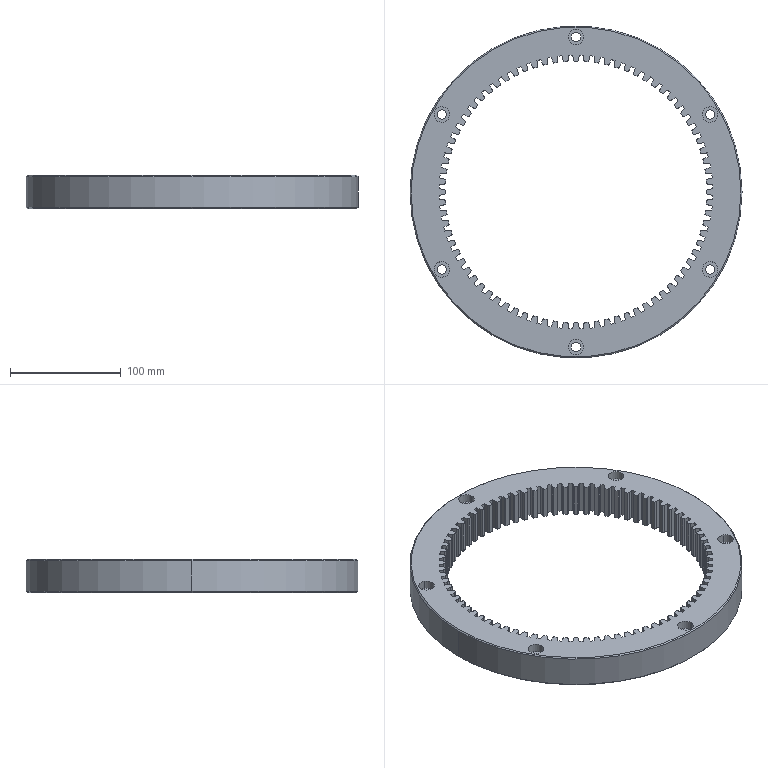Part | Creo | features PROTRUSION 81, CUT 7, CURVE 4, DATUM PLANE 3, PATTERN 2, CHAMFER 1, COORDINATE SYSTEM 1 | 1 solid | 518 faces | box 300 x 300 x 30 mm | volume 727858 mm3 | cylinder 346 | plane 168 | cone 4 | commonest cylinder face diameters 13.456 x160 236.4 x80 247.5 x80 8.5 x12 14 x12 300 x2